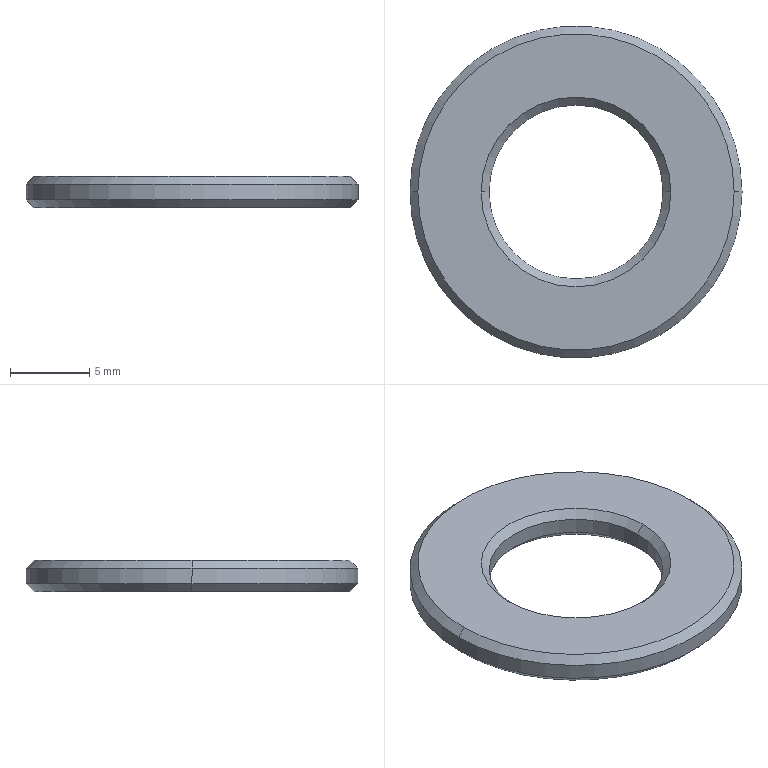Part | SolidWorks | features BaseBody 1 | 1 solid | 14 faces | box 21 x 21 x 2 mm | volume 477.522 mm3 | cone 8 | cylinder 4 | plane 2 | commonest cylinder face diameters 11 x2 21 x2
STEP:
#1=CARTESIAN_POINT('',(-10.,0.,-2.));
#2=VERTEX_POINT('',#1);
#3=CARTESIAN_POINT('',(10.,0.,-2.));
#4=VERTEX_POINT('',#3);
#5=CARTESIAN_POINT('',(0.,0.,-2.));
#6=DIRECTION('',(0.,0.,-1.));
#7=DIRECTION('',(1.,0.,0.));
#8=AXIS2_PLACEMENT_3D('',#5,#6,#7);
#9=CIRCLE('',#8,10.);
#10=EDGE_CURVE('',#2,#4,#9,.T.);
#11=ORIENTED_EDGE('',*,*,#10,.F.);
#12=CARTESIAN_POINT('',(-10.5,0.,-1.5));
#13=VERTEX_POINT('',#12);
#14=CARTESIAN_POINT('',(-10.5,0.,-1.5));
#15=DIRECTION('',(-0.7071,0.,0.7071));
#16=VECTOR('',#15,1000.);
#17=LINE('',#14,#16);
#18=EDGE_CURVE('',#2,#13,#17,.T.);
#19=ORIENTED_EDGE('',*,*,#18,.T.);
#20=CARTESIAN_POINT('',(10.5,0.,-1.5));
#21=VERTEX_POINT('',#20);
#22=CARTESIAN_POINT('',(0.,0.,-1.5));
#23=DIRECTION('',(0.,0.,-1.));
#24=DIRECTION('',(1.,0.,0.));
#25=AXIS2_PLACEMENT_3D('',#22,#23,#24);
#26=CIRCLE('',#25,10.5);
#27=EDGE_CURVE('',#13,#21,#26,.T.);
#28=ORIENTED_EDGE('',*,*,#27,.T.);
#29=CARTESIAN_POINT('',(10.5,0.,-1.5));
#30=DIRECTION('',(0.7071,0.,0.7071));
#31=VECTOR('',#30,1000.);
#32=LINE('',#29,#31);
#33=EDGE_CURVE('',#4,#21,#32,.T.);
#34=ORIENTED_EDGE('',*,*,#33,.F.);
#35=EDGE_LOOP('',(#11,#19,#28,#34));
#36=FACE_OUTER_BOUND('',#35,.T.);
#37=CARTESIAN_POINT('',(0.,0.,-1.5));
#38=DIRECTION('',(0.,0.,1.));
#39=DIRECTION('',(1.,0.,0.));
#40=AXIS2_PLACEMENT_3D('',#37,#38,#39);
#41=CONICAL_SURFACE('',#40,10.5,0.7854);
#42=ADVANCED_FACE('',(#36),#41,.T.);
#43=CARTESIAN_POINT('',(5.5,0.,-1.5));
#44=VERTEX_POINT('',#43);
#45=CARTESIAN_POINT('',(-5.5,0.,-1.5));
#46=VERTEX_POINT('',#45);
#47=CARTESIAN_POINT('',(0.,0.,-1.5));
#48=DIRECTION('',(0.,0.,-1.));
#49=DIRECTION('',(1.,0.,0.));
#50=AXIS2_PLACEMENT_3D('',#47,#48,#49);
#51=CIRCLE('',#50,5.5);
#52=EDGE_CURVE('',#44,#46,#51,.T.);
#53=ORIENTED_EDGE('',*,*,#52,.F.);
#54=CARTESIAN_POINT('',(6.,0.,-2.));
#55=VERTEX_POINT('',#54);
#56=CARTESIAN_POINT('',(6.,0.,-2.));
#57=DIRECTION('',(0.7071,0.,-0.7071));
#58=VECTOR('',#57,1000.);
#59=LINE('',#56,#58);
#60=EDGE_CURVE('',#44,#55,#59,.T.);
#61=ORIENTED_EDGE('',*,*,#60,.T.);
#62=CARTESIAN_POINT('',(-6.,0.,-2.));
#63=VERTEX_POINT('',#62);
#64=CARTESIAN_POINT('',(0.,0.,-2.));
#65=DIRECTION('',(0.,0.,1.));
#66=DIRECTION('',(-1.,0.,0.));
#67=AXIS2_PLACEMENT_3D('',#64,#65,#66);
#68=CIRCLE('',#67,6.);
#69=EDGE_CURVE('',#63,#55,#68,.T.);
#70=ORIENTED_EDGE('',*,*,#69,.F.);
#71=CARTESIAN_POINT('',(-6.,0.,-2.));
#72=DIRECTION('',(-0.7071,0.,-0.7071));
#73=VECTOR('',#72,1000.);
#74=LINE('',#71,#73);
#75=EDGE_CURVE('',#46,#63,#74,.T.);
#76=ORIENTED_EDGE('',*,*,#75,.F.);
#77=EDGE_LOOP('',(#53,#61,#70,#76));
#78=FACE_OUTER_BOUND('',#77,.T.);
#79=CARTESIAN_POINT('',(0.,0.,-2.));
#80=DIRECTION('',(0.,0.,-1.));
#81=DIRECTION('',(-1.,0.,0.));
#82=AXIS2_PLACEMENT_3D('',#79,#80,#81);
#83=CONICAL_SURFACE('',#82,6.,0.7854);
#84=ADVANCED_FACE('',(#78),#83,.F.);
#85=ORIENTED_EDGE('',*,*,#27,.F.);
#86=CARTESIAN_POINT('',(-10.5,0.,-0.5));
#87=VERTEX_POINT('',#86);
#88=CARTESIAN_POINT('',(-10.5,0.,-1.));
#89=DIRECTION('',(0.,0.,1.));
#90=VECTOR('',#89,1000.);
#91=LINE('',#88,#90);
#92=EDGE_CURVE('',#13,#87,#91,.T.);
#93=ORIENTED_EDGE('',*,*,#92,.T.);
#94=CARTESIAN_POINT('',(10.5,0.,-0.5));
#95=VERTEX_POINT('',#94);
#96=CARTESIAN_POINT('',(0.,0.,-0.5));
#97=DIRECTION('',(0.,0.,-1.));
#98=DIRECTION('',(1.,0.,0.));
#99=AXIS2_PLACEMENT_3D('',#96,#97,#98);
#100=CIRCLE('',#99,10.5);
#101=EDGE_CURVE('',#87,#95,#100,.T.);
#102=ORIENTED_EDGE('',*,*,#101,.T.);
#103=CARTESIAN_POINT('',(10.5,0.,-1.));
#104=DIRECTION('',(0.,0.,1.));
#105=VECTOR('',#104,1000.);
#106=LINE('',#103,#105);
#107=EDGE_CURVE('',#21,#95,#106,.T.);
#108=ORIENTED_EDGE('',*,*,#107,.F.);
#109=EDGE_LOOP('',(#85,#93,#102,#108));
#110=FACE_OUTER_BOUND('',#109,.T.);
#111=CARTESIAN_POINT('',(0.,0.,-1.));
#112=DIRECTION('',(0.,0.,1.));
#113=DIRECTION('',(1.,0.,0.));
#114=AXIS2_PLACEMENT_3D('',#111,#112,#113);
#115=CYLINDRICAL_SURFACE('',#114,10.5);
#116=ADVANCED_FACE('',(#110),#115,.T.);
#117=ORIENTED_EDGE('',*,*,#52,.T.);
#118=CARTESIAN_POINT('',(-5.5,0.,-0.5));
#119=VERTEX_POINT('',#118);
#120=CARTESIAN_POINT('',(-5.5,0.,-1.));
#121=DIRECTION('',(0.,0.,1.));
#122=VECTOR('',#121,1000.);
#123=LINE('',#120,#122);
#124=EDGE_CURVE('',#46,#119,#123,.T.);
#125=ORIENTED_EDGE('',*,*,#124,.T.);
#126=CARTESIAN_POINT('',(5.5,0.,-0.5));
#127=VERTEX_POINT('',#126);
#128=CARTESIAN_POINT('',(0.,0.,-0.5));
#129=DIRECTION('',(0.,0.,-1.));
#130=DIRECTION('',(1.,0.,0.));
#131=AXIS2_PLACEMENT_3D('',#128,#129,#130);
#132=CIRCLE('',#131,5.5);
#133=EDGE_CURVE('',#127,#119,#132,.T.);
#134=ORIENTED_EDGE('',*,*,#133,.F.);
#135=CARTESIAN_POINT('',(5.5,0.,-1.));
#136=DIRECTION('',(0.,0.,1.));
#137=VECTOR('',#136,1000.);
#138=LINE('',#135,#137);
#139=EDGE_CURVE('',#44,#127,#138,.T.);
#140=ORIENTED_EDGE('',*,*,#139,.F.);
#141=EDGE_LOOP('',(#117,#125,#134,#140));
#142=FACE_OUTER_BOUND('',#141,.T.);
#143=CARTESIAN_POINT('',(0.,0.,-1.));
#144=DIRECTION('',(0.,0.,1.));
#145=DIRECTION('',(1.,0.,0.));
#146=AXIS2_PLACEMENT_3D('',#143,#144,#145);
#147=CYLINDRICAL_SURFACE('',#146,5.5);
#148=ADVANCED_FACE('',(#142),#147,.F.);
#149=CARTESIAN_POINT('',(-10.,0.,0.));
#150=VERTEX_POINT('',#149);
#151=CARTESIAN_POINT('',(10.,0.,0.));
#152=VERTEX_POINT('',#151);
#153=CARTESIAN_POINT('',(0.,0.,0.));
#154=DIRECTION('',(0.,0.,-1.));
#155=DIRECTION('',(-1.,0.,0.));
#156=AXIS2_PLACEMENT_3D('',#153,#154,#155);
#157=CIRCLE('',#156,10.);
#158=EDGE_CURVE('',#150,#152,#157,.T.);
#159=ORIENTED_EDGE('',*,*,#158,.T.);
#160=CARTESIAN_POINT('',(10.5,0.,-0.5));
#161=DIRECTION('',(0.7071,0.,-0.7071));
#162=VECTOR('',#161,1000.);
#163=LINE('',#160,#162);
#164=EDGE_CURVE('',#152,#95,#163,.T.);
#165=ORIENTED_EDGE('',*,*,#164,.T.);
#166=ORIENTED_EDGE('',*,*,#101,.F.);
#167=CARTESIAN_POINT('',(-10.5,0.,-0.5));
#168=DIRECTION('',(-0.7071,0.,-0.7071));
#169=VECTOR('',#168,1000.);
#170=LINE('',#167,#169);
#171=EDGE_CURVE('',#150,#87,#170,.T.);
#172=ORIENTED_EDGE('',*,*,#171,.F.);
#173=EDGE_LOOP('',(#159,#165,#166,#172));
#174=FACE_OUTER_BOUND('',#173,.T.);
#175=CARTESIAN_POINT('',(0.,0.,-0.5));
#176=DIRECTION('',(0.,0.,-1.));
#177=DIRECTION('',(-1.,0.,0.));
#178=AXIS2_PLACEMENT_3D('',#175,#176,#177);
#179=CONICAL_SURFACE('',#178,10.5,0.7854);
#180=ADVANCED_FACE('',(#174),#179,.T.);
#181=ORIENTED_EDGE('',*,*,#133,.T.);
#182=CARTESIAN_POINT('',(-6.,0.,0.));
#183=VERTEX_POINT('',#182);
#184=CARTESIAN_POINT('',(-6.,0.,0.));
#185=DIRECTION('',(-0.7071,0.,0.7071));
#186=VECTOR('',#185,1000.);
#187=LINE('',#184,#186);
#188=EDGE_CURVE('',#119,#183,#187,.T.);
#189=ORIENTED_EDGE('',*,*,#188,.T.);
#190=CARTESIAN_POINT('',(6.,0.,0.));
#191=VERTEX_POINT('',#190);
#192=CARTESIAN_POINT('',(0.,0.,0.));
#193=DIRECTION('',(0.,0.,-1.));
#194=DIRECTION('',(1.,0.,0.));
#195=AXIS2_PLACEMENT_3D('',#192,#193,#194);
#196=CIRCLE('',#195,6.);
#197=EDGE_CURVE('',#191,#183,#196,.T.);
#198=ORIENTED_EDGE('',*,*,#197,.F.);
#199=CARTESIAN_POINT('',(6.,0.,0.));
#200=DIRECTION('',(0.7071,0.,0.7071));
#201=VECTOR('',#200,1000.);
#202=LINE('',#199,#201);
#203=EDGE_CURVE('',#127,#191,#202,.T.);
#204=ORIENTED_EDGE('',*,*,#203,.F.);
#205=EDGE_LOOP('',(#181,#189,#198,#204));
#206=FACE_OUTER_BOUND('',#205,.T.);
#207=CARTESIAN_POINT('',(0.,0.,0.));
#208=DIRECTION('',(0.,0.,1.));
#209=DIRECTION('',(1.,0.,0.));
#210=AXIS2_PLACEMENT_3D('',#207,#208,#209);
#211=CONICAL_SURFACE('',#210,6.,0.7854);
#212=ADVANCED_FACE('',(#206),#211,.F.);
#213=CARTESIAN_POINT('',(0.,0.,-2.));
#214=DIRECTION('',(0.,0.,-1.));
#215=DIRECTION('',(1.,0.,0.));
#216=AXIS2_PLACEMENT_3D('',#213,#214,#215);
#217=CIRCLE('',#216,10.);
#218=EDGE_CURVE('',#4,#2,#217,.T.);
#219=ORIENTED_EDGE('',*,*,#218,.T.);
#220=ORIENTED_EDGE('',*,*,#10,.T.);
#221=EDGE_LOOP('',(#219,#220));
#222=FACE_OUTER_BOUND('',#221,.T.);
#223=ORIENTED_EDGE('',*,*,#69,.T.);
#224=CARTESIAN_POINT('',(0.,0.,-2.));
#225=DIRECTION('',(0.,0.,1.));
#226=DIRECTION('',(-1.,0.,0.));
#227=AXIS2_PLACEMENT_3D('',#224,#225,#226);
#228=CIRCLE('',#227,6.);
#229=EDGE_CURVE('',#55,#63,#228,.T.);
#230=ORIENTED_EDGE('',*,*,#229,.T.);
#231=EDGE_LOOP('',(#223,#230));
#232=FACE_BOUND('',#231,.T.);
#233=CARTESIAN_POINT('',(5.,0.,-2.));
#234=DIRECTION('',(0.,0.,-1.));
#235=DIRECTION('',(-1.,0.,0.));
#236=AXIS2_PLACEMENT_3D('',#233,#234,#235);
#237=PLANE('',#236);
#238=ADVANCED_FACE('',(#222,#232),#237,.T.);
#239=ORIENTED_EDGE('',*,*,#18,.F.);
#240=ORIENTED_EDGE('',*,*,#218,.F.);
#241=ORIENTED_EDGE('',*,*,#33,.T.);
#242=CARTESIAN_POINT('',(0.,0.,-1.5));
#243=DIRECTION('',(0.,0.,-1.));
#244=DIRECTION('',(1.,0.,0.));
#245=AXIS2_PLACEMENT_3D('',#242,#243,#244);
#246=CIRCLE('',#245,10.5);
#247=EDGE_CURVE('',#21,#13,#246,.T.);
#248=ORIENTED_EDGE('',*,*,#247,.T.);
#249=EDGE_LOOP('',(#239,#240,#241,#248));
#250=FACE_OUTER_BOUND('',#249,.T.);
#251=CARTESIAN_POINT('',(0.,0.,-1.5));
#252=DIRECTION('',(0.,0.,1.));
#253=DIRECTION('',(1.,0.,0.));
#254=AXIS2_PLACEMENT_3D('',#251,#252,#253);
#255=CONICAL_SURFACE('',#254,10.5,0.7854);
#256=ADVANCED_FACE('',(#250),#255,.T.);
#257=ORIENTED_EDGE('',*,*,#60,.F.);
#258=CARTESIAN_POINT('',(0.,0.,-1.5));
#259=DIRECTION('',(0.,0.,-1.));
#260=DIRECTION('',(1.,0.,0.));
#261=AXIS2_PLACEMENT_3D('',#258,#259,#260);
#262=CIRCLE('',#261,5.5);
#263=EDGE_CURVE('',#46,#44,#262,.T.);
#264=ORIENTED_EDGE('',*,*,#263,.F.);
#265=ORIENTED_EDGE('',*,*,#75,.T.);
#266=ORIENTED_EDGE('',*,*,#229,.F.);
#267=EDGE_LOOP('',(#257,#264,#265,#266));
#268=FACE_OUTER_BOUND('',#267,.T.);
#269=CARTESIAN_POINT('',(0.,0.,-2.));
#270=DIRECTION('',(0.,0.,-1.));
#271=DIRECTION('',(-1.,0.,0.));
#272=AXIS2_PLACEMENT_3D('',#269,#270,#271);
#273=CONICAL_SURFACE('',#272,6.,0.7854);
#274=ADVANCED_FACE('',(#268),#273,.F.);
#275=ORIENTED_EDGE('',*,*,#92,.F.);
#276=ORIENTED_EDGE('',*,*,#247,.F.);
#277=ORIENTED_EDGE('',*,*,#107,.T.);
#278=CARTESIAN_POINT('',(0.,0.,-0.5));
#279=DIRECTION('',(0.,0.,-1.));
#280=DIRECTION('',(1.,0.,0.));
#281=AXIS2_PLACEMENT_3D('',#278,#279,#280);
#282=CIRCLE('',#281,10.5);
#283=EDGE_CURVE('',#95,#87,#282,.T.);
#284=ORIENTED_EDGE('',*,*,#283,.T.);
#285=EDGE_LOOP('',(#275,#276,#277,#284));
#286=FACE_OUTER_BOUND('',#285,.T.);
#287=CARTESIAN_POINT('',(0.,0.,-1.));
#288=DIRECTION('',(0.,0.,1.));
#289=DIRECTION('',(1.,0.,0.));
#290=AXIS2_PLACEMENT_3D('',#287,#288,#289);
#291=CYLINDRICAL_SURFACE('',#290,10.5);
#292=ADVANCED_FACE('',(#286),#291,.T.);
#293=ORIENTED_EDGE('',*,*,#124,.F.);
#294=ORIENTED_EDGE('',*,*,#263,.T.);
#295=ORIENTED_EDGE('',*,*,#139,.T.);
#296=CARTESIAN_POINT('',(0.,0.,-0.5));
#297=DIRECTION('',(0.,0.,-1.));
#298=DIRECTION('',(1.,0.,0.));
#299=AXIS2_PLACEMENT_3D('',#296,#297,#298);
#300=CIRCLE('',#299,5.5);
#301=EDGE_CURVE('',#119,#127,#300,.T.);
#302=ORIENTED_EDGE('',*,*,#301,.F.);
#303=EDGE_LOOP('',(#293,#294,#295,#302));
#304=FACE_OUTER_BOUND('',#303,.T.);
#305=CARTESIAN_POINT('',(0.,0.,-1.));
#306=DIRECTION('',(0.,0.,1.));
#307=DIRECTION('',(1.,0.,0.));
#308=AXIS2_PLACEMENT_3D('',#305,#306,#307);
#309=CYLINDRICAL_SURFACE('',#308,5.5);
#310=ADVANCED_FACE('',(#304),#309,.F.);
#311=ORIENTED_EDGE('',*,*,#164,.F.);
#312=CARTESIAN_POINT('',(0.,0.,0.));
#313=DIRECTION('',(0.,0.,-1.));
#314=DIRECTION('',(-1.,0.,0.));
#315=AXIS2_PLACEMENT_3D('',#312,#313,#314);
#316=CIRCLE('',#315,10.);
#317=EDGE_CURVE('',#152,#150,#316,.T.);
#318=ORIENTED_EDGE('',*,*,#317,.T.);
#319=ORIENTED_EDGE('',*,*,#171,.T.);
#320=ORIENTED_EDGE('',*,*,#283,.F.);
#321=EDGE_LOOP('',(#311,#318,#319,#320));
#322=FACE_OUTER_BOUND('',#321,.T.);
#323=CARTESIAN_POINT('',(0.,0.,-0.5));
#324=DIRECTION('',(0.,0.,-1.));
#325=DIRECTION('',(-1.,0.,0.));
#326=AXIS2_PLACEMENT_3D('',#323,#324,#325);
#327=CONICAL_SURFACE('',#326,10.5,0.7854);
#328=ADVANCED_FACE('',(#322),#327,.T.);
#329=ORIENTED_EDGE('',*,*,#188,.F.);
#330=ORIENTED_EDGE('',*,*,#301,.T.);
#331=ORIENTED_EDGE('',*,*,#203,.T.);
#332=CARTESIAN_POINT('',(0.,0.,0.));
#333=DIRECTION('',(0.,0.,-1.));
#334=DIRECTION('',(1.,0.,0.));
#335=AXIS2_PLACEMENT_3D('',#332,#333,#334);
#336=CIRCLE('',#335,6.);
#337=EDGE_CURVE('',#183,#191,#336,.T.);
#338=ORIENTED_EDGE('',*,*,#337,.F.);
#339=EDGE_LOOP('',(#329,#330,#331,#338));
#340=FACE_OUTER_BOUND('',#339,.T.);
#341=CARTESIAN_POINT('',(0.,0.,0.));
#342=DIRECTION('',(0.,0.,1.));
#343=DIRECTION('',(1.,0.,0.));
#344=AXIS2_PLACEMENT_3D('',#341,#342,#343);
#345=CONICAL_SURFACE('',#344,6.,0.7854);
#346=ADVANCED_FACE('',(#340),#345,.F.);
#347=ORIENTED_EDGE('',*,*,#158,.F.);
#348=ORIENTED_EDGE('',*,*,#317,.F.);
#349=EDGE_LOOP('',(#347,#348));
#350=FACE_OUTER_BOUND('',#349,.T.);
#351=ORIENTED_EDGE('',*,*,#197,.T.);
#352=ORIENTED_EDGE('',*,*,#337,.T.);
#353=EDGE_LOOP('',(#351,#352));
#354=FACE_BOUND('',#353,.T.);
#355=CARTESIAN_POINT('',(5.,0.,0.));
#356=DIRECTION('',(0.,0.,1.));
#357=DIRECTION('',(1.,0.,0.));
#358=AXIS2_PLACEMENT_3D('',#355,#356,#357);
#359=PLANE('',#358);
#360=ADVANCED_FACE('',(#350,#354),#359,.T.);
#361=CLOSED_SHELL('',(#42,#84,#116,#148,#180,#212,#238,#256,#274,#292,#310,#328,#346,#360));
#362=MANIFOLD_SOLID_BREP('',#361);
#363=CARTESIAN_POINT('',(0.,0.,0.));
#364=DIRECTION('',(0.,0.,1.));
#365=DIRECTION('',(1.,0.,0.));
#366=AXIS2_PLACEMENT_3D('',#363,#364,#365);
#367=(LENGTH_UNIT()NAMED_UNIT(*)SI_UNIT(.MILLI.,.METRE.));
#368=UNCERTAINTY_MEASURE_WITH_UNIT(LENGTH_MEASURE(0.00001),#367,'','');
#369=(NAMED_UNIT(*)PLANE_ANGLE_UNIT()SI_UNIT($,.RADIAN.));
#370=(NAMED_UNIT(*)SI_UNIT($,.STERADIAN.)SOLID_ANGLE_UNIT());
#371=(GEOMETRIC_REPRESENTATION_CONTEXT(3)GLOBAL_UNCERTAINTY_ASSIGNED_CONTEXT((#368))GLOBAL_UNIT_ASSIGNED_CONTEXT((#367,#369,#370))REPRESENTATION_CONTEXT('',''));
#372=ADVANCED_BREP_SHAPE_REPRESENTATION('',(#362,#366),#371);